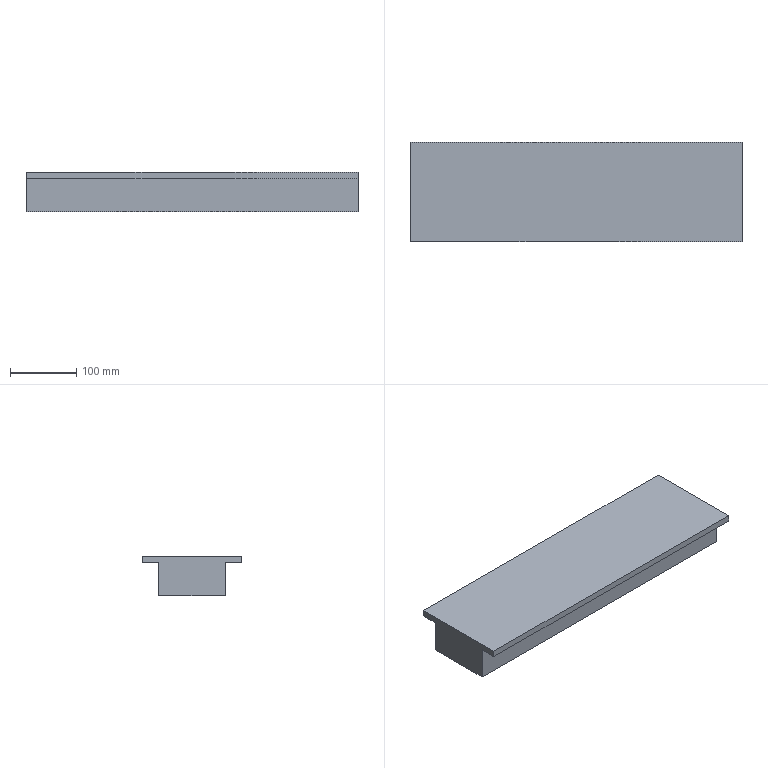Part | SolidWorks | features Extrusion 1, ICE 1 | 1 solid | 10 faces | box 500 x 150 x 60 mm | volume 3250000 mm3 | plane 10
STEP:
#1=CARTESIAN_POINT('',(250.,-50.,0.));
#2=VERTEX_POINT('',#1);
#3=CARTESIAN_POINT('',(-250.,-50.,0.));
#4=VERTEX_POINT('',#3);
#5=CARTESIAN_POINT('',(250.,-50.,0.));
#6=DIRECTION('',(-1.,0.,0.));
#7=VECTOR('',#6,1000.);
#8=LINE('',#5,#7);
#9=EDGE_CURVE('',#2,#4,#8,.T.);
#10=ORIENTED_EDGE('',*,*,#9,.F.);
#11=CARTESIAN_POINT('',(250.,-75.,0.));
#12=VERTEX_POINT('',#11);
#13=CARTESIAN_POINT('',(250.,75.,0.));
#14=DIRECTION('',(0.,1.,0.));
#15=VECTOR('',#14,1000.);
#16=LINE('',#13,#15);
#17=EDGE_CURVE('',#12,#2,#16,.T.);
#18=ORIENTED_EDGE('',*,*,#17,.F.);
#19=CARTESIAN_POINT('',(-250.,-75.,0.));
#20=VERTEX_POINT('',#19);
#21=CARTESIAN_POINT('',(-250.,-75.,0.));
#22=DIRECTION('',(1.,0.,0.));
#23=VECTOR('',#22,1000.);
#24=LINE('',#21,#23);
#25=EDGE_CURVE('',#20,#12,#24,.T.);
#26=ORIENTED_EDGE('',*,*,#25,.F.);
#27=CARTESIAN_POINT('',(-250.,75.,0.));
#28=DIRECTION('',(0.,-1.,0.));
#29=VECTOR('',#28,1000.);
#30=LINE('',#27,#29);
#31=EDGE_CURVE('',#4,#20,#30,.T.);
#32=ORIENTED_EDGE('',*,*,#31,.F.);
#33=EDGE_LOOP('',(#10,#18,#26,#32));
#34=FACE_OUTER_BOUND('',#33,.T.);
#35=CARTESIAN_POINT('',(0.,0.,0.));
#36=DIRECTION('',(0.,0.,1.));
#37=DIRECTION('',(1.,0.,0.));
#38=AXIS2_PLACEMENT_3D('',#35,#36,#37);
#39=PLANE('',#38);
#40=ADVANCED_FACE('',(#34),#39,.F.);
#41=CARTESIAN_POINT('',(-250.,50.,0.));
#42=VERTEX_POINT('',#41);
#43=CARTESIAN_POINT('',(250.,50.,0.));
#44=VERTEX_POINT('',#43);
#45=CARTESIAN_POINT('',(250.,50.,0.));
#46=DIRECTION('',(1.,0.,0.));
#47=VECTOR('',#46,1000.);
#48=LINE('',#45,#47);
#49=EDGE_CURVE('',#42,#44,#48,.T.);
#50=ORIENTED_EDGE('',*,*,#49,.F.);
#51=CARTESIAN_POINT('',(-250.,75.,0.));
#52=VERTEX_POINT('',#51);
#53=CARTESIAN_POINT('',(-250.,75.,0.));
#54=DIRECTION('',(0.,-1.,0.));
#55=VECTOR('',#54,1000.);
#56=LINE('',#53,#55);
#57=EDGE_CURVE('',#52,#42,#56,.T.);
#58=ORIENTED_EDGE('',*,*,#57,.F.);
#59=CARTESIAN_POINT('',(250.,75.,0.));
#60=VERTEX_POINT('',#59);
#61=CARTESIAN_POINT('',(-250.,75.,0.));
#62=DIRECTION('',(-1.,0.,0.));
#63=VECTOR('',#62,1000.);
#64=LINE('',#61,#63);
#65=EDGE_CURVE('',#60,#52,#64,.T.);
#66=ORIENTED_EDGE('',*,*,#65,.F.);
#67=CARTESIAN_POINT('',(250.,75.,0.));
#68=DIRECTION('',(0.,1.,0.));
#69=VECTOR('',#68,1000.);
#70=LINE('',#67,#69);
#71=EDGE_CURVE('',#44,#60,#70,.T.);
#72=ORIENTED_EDGE('',*,*,#71,.F.);
#73=EDGE_LOOP('',(#50,#58,#66,#72));
#74=FACE_OUTER_BOUND('',#73,.T.);
#75=CARTESIAN_POINT('',(0.,0.,0.));
#76=DIRECTION('',(0.,0.,1.));
#77=DIRECTION('',(1.,0.,0.));
#78=AXIS2_PLACEMENT_3D('',#75,#76,#77);
#79=PLANE('',#78);
#80=ADVANCED_FACE('',(#74),#79,.F.);
#81=ORIENTED_EDGE('',*,*,#17,.T.);
#82=CARTESIAN_POINT('',(250.,-50.,-50.));
#83=VERTEX_POINT('',#82);
#84=CARTESIAN_POINT('',(250.,-50.,-50.));
#85=DIRECTION('',(0.,0.,1.));
#86=VECTOR('',#85,1000.);
#87=LINE('',#84,#86);
#88=EDGE_CURVE('',#83,#2,#87,.T.);
#89=ORIENTED_EDGE('',*,*,#88,.F.);
#90=CARTESIAN_POINT('',(250.,50.,-50.));
#91=VERTEX_POINT('',#90);
#92=CARTESIAN_POINT('',(250.,50.,-50.));
#93=DIRECTION('',(0.,-1.,0.));
#94=VECTOR('',#93,1000.);
#95=LINE('',#92,#94);
#96=EDGE_CURVE('',#91,#83,#95,.T.);
#97=ORIENTED_EDGE('',*,*,#96,.F.);
#98=CARTESIAN_POINT('',(250.,50.,-50.));
#99=DIRECTION('',(0.,0.,1.));
#100=VECTOR('',#99,1000.);
#101=LINE('',#98,#100);
#102=EDGE_CURVE('',#91,#44,#101,.T.);
#103=ORIENTED_EDGE('',*,*,#102,.T.);
#104=ORIENTED_EDGE('',*,*,#71,.T.);
#105=CARTESIAN_POINT('',(250.,75.,10.));
#106=VERTEX_POINT('',#105);
#107=CARTESIAN_POINT('',(250.,75.,10.));
#108=DIRECTION('',(0.,0.,-1.));
#109=VECTOR('',#108,1000.);
#110=LINE('',#107,#109);
#111=EDGE_CURVE('',#106,#60,#110,.T.);
#112=ORIENTED_EDGE('',*,*,#111,.F.);
#113=CARTESIAN_POINT('',(250.,-75.,10.));
#114=VERTEX_POINT('',#113);
#115=CARTESIAN_POINT('',(250.,75.,10.));
#116=DIRECTION('',(0.,1.,0.));
#117=VECTOR('',#116,1000.);
#118=LINE('',#115,#117);
#119=EDGE_CURVE('',#114,#106,#118,.T.);
#120=ORIENTED_EDGE('',*,*,#119,.F.);
#121=CARTESIAN_POINT('',(250.,-75.,10.));
#122=DIRECTION('',(0.,0.,-1.));
#123=VECTOR('',#122,1000.);
#124=LINE('',#121,#123);
#125=EDGE_CURVE('',#114,#12,#124,.T.);
#126=ORIENTED_EDGE('',*,*,#125,.T.);
#127=EDGE_LOOP('',(#81,#89,#97,#103,#104,#112,#120,#126));
#128=FACE_OUTER_BOUND('',#127,.T.);
#129=CARTESIAN_POINT('',(250.,75.,10.));
#130=DIRECTION('',(-1.,0.,0.));
#131=DIRECTION('',(0.,-1.,0.));
#132=AXIS2_PLACEMENT_3D('',#129,#130,#131);
#133=PLANE('',#132);
#134=ADVANCED_FACE('',(#128),#133,.F.);
#135=ORIENTED_EDGE('',*,*,#65,.T.);
#136=CARTESIAN_POINT('',(-250.,75.,10.));
#137=VERTEX_POINT('',#136);
#138=CARTESIAN_POINT('',(-250.,75.,10.));
#139=DIRECTION('',(0.,0.,-1.));
#140=VECTOR('',#139,1000.);
#141=LINE('',#138,#140);
#142=EDGE_CURVE('',#137,#52,#141,.T.);
#143=ORIENTED_EDGE('',*,*,#142,.F.);
#144=CARTESIAN_POINT('',(-250.,75.,10.));
#145=DIRECTION('',(-1.,0.,0.));
#146=VECTOR('',#145,1000.);
#147=LINE('',#144,#146);
#148=EDGE_CURVE('',#106,#137,#147,.T.);
#149=ORIENTED_EDGE('',*,*,#148,.F.);
#150=ORIENTED_EDGE('',*,*,#111,.T.);
#151=EDGE_LOOP('',(#135,#143,#149,#150));
#152=FACE_OUTER_BOUND('',#151,.T.);
#153=CARTESIAN_POINT('',(-250.,75.,10.));
#154=DIRECTION('',(0.,-1.,0.));
#155=DIRECTION('',(0.,0.,-1.));
#156=AXIS2_PLACEMENT_3D('',#153,#154,#155);
#157=PLANE('',#156);
#158=ADVANCED_FACE('',(#152),#157,.F.);
#159=ORIENTED_EDGE('',*,*,#57,.T.);
#160=CARTESIAN_POINT('',(-250.,50.,-50.));
#161=VERTEX_POINT('',#160);
#162=CARTESIAN_POINT('',(-250.,50.,-50.));
#163=DIRECTION('',(0.,0.,1.));
#164=VECTOR('',#163,1000.);
#165=LINE('',#162,#164);
#166=EDGE_CURVE('',#161,#42,#165,.T.);
#167=ORIENTED_EDGE('',*,*,#166,.F.);
#168=CARTESIAN_POINT('',(-250.,-50.,-50.));
#169=VERTEX_POINT('',#168);
#170=CARTESIAN_POINT('',(-250.,50.,-50.));
#171=DIRECTION('',(0.,1.,0.));
#172=VECTOR('',#171,1000.);
#173=LINE('',#170,#172);
#174=EDGE_CURVE('',#169,#161,#173,.T.);
#175=ORIENTED_EDGE('',*,*,#174,.F.);
#176=CARTESIAN_POINT('',(-250.,-50.,-50.));
#177=DIRECTION('',(0.,0.,1.));
#178=VECTOR('',#177,1000.);
#179=LINE('',#176,#178);
#180=EDGE_CURVE('',#169,#4,#179,.T.);
#181=ORIENTED_EDGE('',*,*,#180,.T.);
#182=ORIENTED_EDGE('',*,*,#31,.T.);
#183=CARTESIAN_POINT('',(-250.,-75.,10.));
#184=VERTEX_POINT('',#183);
#185=CARTESIAN_POINT('',(-250.,-75.,10.));
#186=DIRECTION('',(0.,0.,-1.));
#187=VECTOR('',#186,1000.);
#188=LINE('',#185,#187);
#189=EDGE_CURVE('',#184,#20,#188,.T.);
#190=ORIENTED_EDGE('',*,*,#189,.F.);
#191=CARTESIAN_POINT('',(-250.,75.,10.));
#192=DIRECTION('',(0.,-1.,0.));
#193=VECTOR('',#192,1000.);
#194=LINE('',#191,#193);
#195=EDGE_CURVE('',#137,#184,#194,.T.);
#196=ORIENTED_EDGE('',*,*,#195,.F.);
#197=ORIENTED_EDGE('',*,*,#142,.T.);
#198=EDGE_LOOP('',(#159,#167,#175,#181,#182,#190,#196,#197));
#199=FACE_OUTER_BOUND('',#198,.T.);
#200=CARTESIAN_POINT('',(-250.,75.,10.));
#201=DIRECTION('',(1.,0.,0.));
#202=DIRECTION('',(0.,1.,0.));
#203=AXIS2_PLACEMENT_3D('',#200,#201,#202);
#204=PLANE('',#203);
#205=ADVANCED_FACE('',(#199),#204,.F.);
#206=ORIENTED_EDGE('',*,*,#25,.T.);
#207=ORIENTED_EDGE('',*,*,#125,.F.);
#208=CARTESIAN_POINT('',(-250.,-75.,10.));
#209=DIRECTION('',(1.,0.,0.));
#210=VECTOR('',#209,1000.);
#211=LINE('',#208,#210);
#212=EDGE_CURVE('',#184,#114,#211,.T.);
#213=ORIENTED_EDGE('',*,*,#212,.F.);
#214=ORIENTED_EDGE('',*,*,#189,.T.);
#215=EDGE_LOOP('',(#206,#207,#213,#214));
#216=FACE_OUTER_BOUND('',#215,.T.);
#217=CARTESIAN_POINT('',(-250.,-75.,10.));
#218=DIRECTION('',(0.,1.,0.));
#219=DIRECTION('',(0.,0.,1.));
#220=AXIS2_PLACEMENT_3D('',#217,#218,#219);
#221=PLANE('',#220);
#222=ADVANCED_FACE('',(#216),#221,.F.);
#223=ORIENTED_EDGE('',*,*,#119,.T.);
#224=ORIENTED_EDGE('',*,*,#148,.T.);
#225=ORIENTED_EDGE('',*,*,#195,.T.);
#226=ORIENTED_EDGE('',*,*,#212,.T.);
#227=EDGE_LOOP('',(#223,#224,#225,#226));
#228=FACE_OUTER_BOUND('',#227,.T.);
#229=CARTESIAN_POINT('',(0.,0.,10.));
#230=DIRECTION('',(0.,0.,1.));
#231=DIRECTION('',(1.,0.,0.));
#232=AXIS2_PLACEMENT_3D('',#229,#230,#231);
#233=PLANE('',#232);
#234=ADVANCED_FACE('',(#228),#233,.T.);
#235=ORIENTED_EDGE('',*,*,#49,.T.);
#236=ORIENTED_EDGE('',*,*,#102,.F.);
#237=CARTESIAN_POINT('',(250.,50.,-50.));
#238=DIRECTION('',(1.,0.,0.));
#239=VECTOR('',#238,1000.);
#240=LINE('',#237,#239);
#241=EDGE_CURVE('',#161,#91,#240,.T.);
#242=ORIENTED_EDGE('',*,*,#241,.F.);
#243=ORIENTED_EDGE('',*,*,#166,.T.);
#244=EDGE_LOOP('',(#235,#236,#242,#243));
#245=FACE_OUTER_BOUND('',#244,.T.);
#246=CARTESIAN_POINT('',(250.,50.,-50.));
#247=DIRECTION('',(0.,-1.,0.));
#248=DIRECTION('',(0.,0.,-1.));
#249=AXIS2_PLACEMENT_3D('',#246,#247,#248);
#250=PLANE('',#249);
#251=ADVANCED_FACE('',(#245),#250,.F.);
#252=ORIENTED_EDGE('',*,*,#9,.T.);
#253=ORIENTED_EDGE('',*,*,#180,.F.);
#254=CARTESIAN_POINT('',(250.,-50.,-50.));
#255=DIRECTION('',(-1.,0.,0.));
#256=VECTOR('',#255,1000.);
#257=LINE('',#254,#256);
#258=EDGE_CURVE('',#83,#169,#257,.T.);
#259=ORIENTED_EDGE('',*,*,#258,.F.);
#260=ORIENTED_EDGE('',*,*,#88,.T.);
#261=EDGE_LOOP('',(#252,#253,#259,#260));
#262=FACE_OUTER_BOUND('',#261,.T.);
#263=CARTESIAN_POINT('',(250.,-50.,-50.));
#264=DIRECTION('',(0.,1.,0.));
#265=DIRECTION('',(0.,0.,1.));
#266=AXIS2_PLACEMENT_3D('',#263,#264,#265);
#267=PLANE('',#266);
#268=ADVANCED_FACE('',(#262),#267,.F.);
#269=ORIENTED_EDGE('',*,*,#174,.T.);
#270=ORIENTED_EDGE('',*,*,#241,.T.);
#271=ORIENTED_EDGE('',*,*,#96,.T.);
#272=ORIENTED_EDGE('',*,*,#258,.T.);
#273=EDGE_LOOP('',(#269,#270,#271,#272));
#274=FACE_OUTER_BOUND('',#273,.T.);
#275=CARTESIAN_POINT('',(0.,0.,-50.));
#276=DIRECTION('',(0.,0.,-1.));
#277=DIRECTION('',(-1.,0.,0.));
#278=AXIS2_PLACEMENT_3D('',#275,#276,#277);
#279=PLANE('',#278);
#280=ADVANCED_FACE('',(#274),#279,.T.);
#281=CLOSED_SHELL('',(#40,#80,#134,#158,#205,#222,#234,#251,#268,#280));
#282=MANIFOLD_SOLID_BREP('',#281);
#283=CARTESIAN_POINT('',(0.,0.,0.));
#284=DIRECTION('',(0.,0.,1.));
#285=DIRECTION('',(1.,0.,0.));
#286=AXIS2_PLACEMENT_3D('',#283,#284,#285);
#287=(LENGTH_UNIT()NAMED_UNIT(*)SI_UNIT(.MILLI.,.METRE.));
#288=UNCERTAINTY_MEASURE_WITH_UNIT(LENGTH_MEASURE(0.00001),#287,'','');
#289=(NAMED_UNIT(*)PLANE_ANGLE_UNIT()SI_UNIT($,.RADIAN.));
#290=(NAMED_UNIT(*)SI_UNIT($,.STERADIAN.)SOLID_ANGLE_UNIT());
#291=(GEOMETRIC_REPRESENTATION_CONTEXT(3)GLOBAL_UNCERTAINTY_ASSIGNED_CONTEXT((#288))GLOBAL_UNIT_ASSIGNED_CONTEXT((#287,#289,#290))REPRESENTATION_CONTEXT('',''));
#292=ADVANCED_BREP_SHAPE_REPRESENTATION('',(#282,#286),#291);